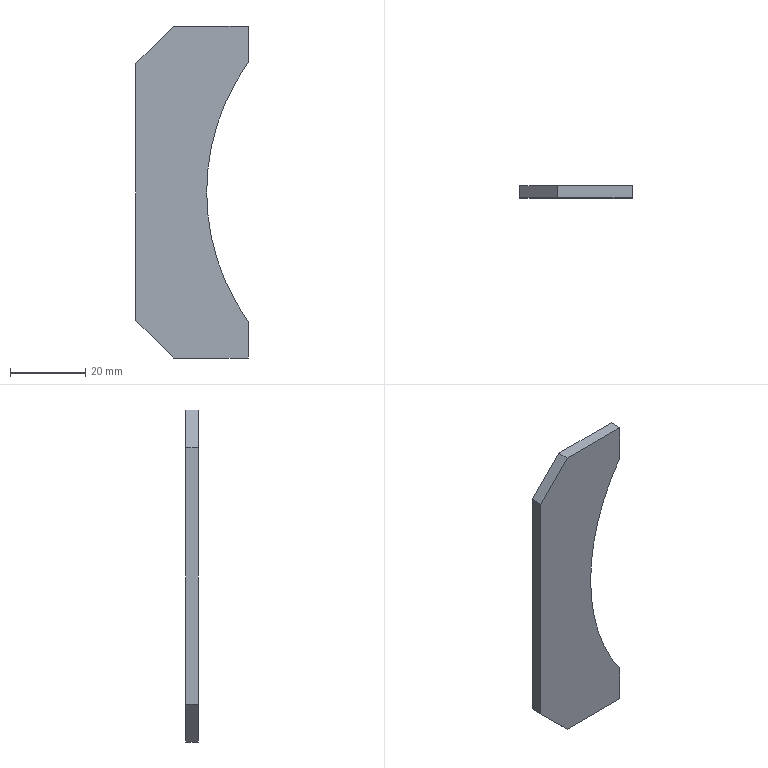Part | SolidWorks | features FlatPattern 1, SMBaseFlange 1, SheetMetal 1 | 1 solid | 10 faces | box 29.8 x 3.2 x 88.1 mm | volume 6438 mm3 | plane 9 | cylinder 1 | commonest cylinder face diameters 118 x1
STEP:
#1=CARTESIAN_POINT('',(0.,0.,9.743));
#2=VERTEX_POINT('',#1);
#3=CARTESIAN_POINT('',(0.,0.,0.));
#4=VERTEX_POINT('',#3);
#5=CARTESIAN_POINT('',(0.,0.,9.743));
#6=DIRECTION('',(0.,0.,-1.));
#7=VECTOR('',#6,1000.);
#8=LINE('',#5,#7);
#9=EDGE_CURVE('',#2,#4,#8,.T.);
#10=ORIENTED_EDGE('',*,*,#9,.F.);
#11=CARTESIAN_POINT('',(0.,-3.2,9.743));
#12=VERTEX_POINT('',#11);
#13=CARTESIAN_POINT('',(0.,-3.2,9.743));
#14=DIRECTION('',(0.,1.,0.));
#15=VECTOR('',#14,1000.);
#16=LINE('',#13,#15);
#17=EDGE_CURVE('',#12,#2,#16,.T.);
#18=ORIENTED_EDGE('',*,*,#17,.F.);
#19=CARTESIAN_POINT('',(0.,-3.2,0.));
#20=VERTEX_POINT('',#19);
#21=CARTESIAN_POINT('',(0.,-3.2,9.743));
#22=DIRECTION('',(0.,0.,-1.));
#23=VECTOR('',#22,1000.);
#24=LINE('',#21,#23);
#25=EDGE_CURVE('',#12,#20,#24,.T.);
#26=ORIENTED_EDGE('',*,*,#25,.T.);
#27=CARTESIAN_POINT('',(0.,-3.2,0.));
#28=DIRECTION('',(0.,1.,0.));
#29=VECTOR('',#28,1000.);
#30=LINE('',#27,#29);
#31=EDGE_CURVE('',#20,#4,#30,.T.);
#32=ORIENTED_EDGE('',*,*,#31,.T.);
#33=EDGE_LOOP('',(#10,#18,#26,#32));
#34=FACE_OUTER_BOUND('',#33,.T.);
#35=CARTESIAN_POINT('',(0.,-3.2,9.743));
#36=DIRECTION('',(1.,0.,0.));
#37=DIRECTION('',(0.,0.,-1.));
#38=AXIS2_PLACEMENT_3D('',#35,#36,#37);
#39=PLANE('',#38);
#40=ADVANCED_FACE('',(#34),#39,.T.);
#41=CARTESIAN_POINT('',(0.,0.,78.357));
#42=VERTEX_POINT('',#41);
#43=CARTESIAN_POINT('',(48.,0.,44.05));
#44=DIRECTION('',(0.,-1.,0.));
#45=DIRECTION('',(0.,0.,1.));
#46=AXIS2_PLACEMENT_3D('',#43,#44,#45);
#47=CIRCLE('',#46,59.);
#48=EDGE_CURVE('',#42,#2,#47,.T.);
#49=ORIENTED_EDGE('',*,*,#48,.F.);
#50=CARTESIAN_POINT('',(0.,-3.2,78.357));
#51=VERTEX_POINT('',#50);
#52=CARTESIAN_POINT('',(0.,-3.2,78.357));
#53=DIRECTION('',(0.,1.,0.));
#54=VECTOR('',#53,1000.);
#55=LINE('',#52,#54);
#56=EDGE_CURVE('',#51,#42,#55,.T.);
#57=ORIENTED_EDGE('',*,*,#56,.F.);
#58=CARTESIAN_POINT('',(48.,-3.2,44.05));
#59=DIRECTION('',(0.,-1.,0.));
#60=DIRECTION('',(0.,0.,1.));
#61=AXIS2_PLACEMENT_3D('',#58,#59,#60);
#62=CIRCLE('',#61,59.);
#63=EDGE_CURVE('',#51,#12,#62,.T.);
#64=ORIENTED_EDGE('',*,*,#63,.T.);
#65=ORIENTED_EDGE('',*,*,#17,.T.);
#66=EDGE_LOOP('',(#49,#57,#64,#65));
#67=FACE_OUTER_BOUND('',#66,.T.);
#68=CARTESIAN_POINT('',(48.,-3.2,44.05));
#69=DIRECTION('',(0.,1.,0.));
#70=DIRECTION('',(0.,0.,1.));
#71=AXIS2_PLACEMENT_3D('',#68,#69,#70);
#72=CYLINDRICAL_SURFACE('',#71,59.);
#73=ADVANCED_FACE('',(#67),#72,.F.);
#74=CARTESIAN_POINT('',(0.,0.,88.1));
#75=VERTEX_POINT('',#74);
#76=CARTESIAN_POINT('',(0.,0.,88.1));
#77=DIRECTION('',(0.,0.,-1.));
#78=VECTOR('',#77,1000.);
#79=LINE('',#76,#78);
#80=EDGE_CURVE('',#75,#42,#79,.T.);
#81=ORIENTED_EDGE('',*,*,#80,.F.);
#82=CARTESIAN_POINT('',(0.,-3.2,88.1));
#83=VERTEX_POINT('',#82);
#84=CARTESIAN_POINT('',(0.,-3.2,88.1));
#85=DIRECTION('',(0.,1.,0.));
#86=VECTOR('',#85,1000.);
#87=LINE('',#84,#86);
#88=EDGE_CURVE('',#83,#75,#87,.T.);
#89=ORIENTED_EDGE('',*,*,#88,.F.);
#90=CARTESIAN_POINT('',(0.,-3.2,88.1));
#91=DIRECTION('',(0.,0.,-1.));
#92=VECTOR('',#91,1000.);
#93=LINE('',#90,#92);
#94=EDGE_CURVE('',#83,#51,#93,.T.);
#95=ORIENTED_EDGE('',*,*,#94,.T.);
#96=ORIENTED_EDGE('',*,*,#56,.T.);
#97=EDGE_LOOP('',(#81,#89,#95,#96));
#98=FACE_OUTER_BOUND('',#97,.T.);
#99=CARTESIAN_POINT('',(0.,-3.2,88.1));
#100=DIRECTION('',(1.,0.,0.));
#101=DIRECTION('',(0.,0.,-1.));
#102=AXIS2_PLACEMENT_3D('',#99,#100,#101);
#103=PLANE('',#102);
#104=ADVANCED_FACE('',(#98),#103,.T.);
#105=CARTESIAN_POINT('',(-19.8,0.,88.1));
#106=VERTEX_POINT('',#105);
#107=CARTESIAN_POINT('',(-19.8,0.,88.1));
#108=DIRECTION('',(1.,0.,0.));
#109=VECTOR('',#108,1000.);
#110=LINE('',#107,#109);
#111=EDGE_CURVE('',#106,#75,#110,.T.);
#112=ORIENTED_EDGE('',*,*,#111,.F.);
#113=CARTESIAN_POINT('',(-19.8,-3.2,88.1));
#114=VERTEX_POINT('',#113);
#115=CARTESIAN_POINT('',(-19.8,-3.2,88.1));
#116=DIRECTION('',(0.,1.,0.));
#117=VECTOR('',#116,1000.);
#118=LINE('',#115,#117);
#119=EDGE_CURVE('',#114,#106,#118,.T.);
#120=ORIENTED_EDGE('',*,*,#119,.F.);
#121=CARTESIAN_POINT('',(-19.8,-3.2,88.1));
#122=DIRECTION('',(1.,0.,0.));
#123=VECTOR('',#122,1000.);
#124=LINE('',#121,#123);
#125=EDGE_CURVE('',#114,#83,#124,.T.);
#126=ORIENTED_EDGE('',*,*,#125,.T.);
#127=ORIENTED_EDGE('',*,*,#88,.T.);
#128=EDGE_LOOP('',(#112,#120,#126,#127));
#129=FACE_OUTER_BOUND('',#128,.T.);
#130=CARTESIAN_POINT('',(-19.8,-3.2,88.1));
#131=DIRECTION('',(0.,0.,1.));
#132=DIRECTION('',(1.,0.,0.));
#133=AXIS2_PLACEMENT_3D('',#130,#131,#132);
#134=PLANE('',#133);
#135=ADVANCED_FACE('',(#129),#134,.T.);
#136=CARTESIAN_POINT('',(-29.8,0.,78.1));
#137=VERTEX_POINT('',#136);
#138=CARTESIAN_POINT('',(-29.8,0.,78.1));
#139=DIRECTION('',(0.7071,0.,0.7071));
#140=VECTOR('',#139,1000.);
#141=LINE('',#138,#140);
#142=EDGE_CURVE('',#137,#106,#141,.T.);
#143=ORIENTED_EDGE('',*,*,#142,.F.);
#144=CARTESIAN_POINT('',(-29.8,-3.2,78.1));
#145=VERTEX_POINT('',#144);
#146=CARTESIAN_POINT('',(-29.8,-3.2,78.1));
#147=DIRECTION('',(0.,1.,0.));
#148=VECTOR('',#147,1000.);
#149=LINE('',#146,#148);
#150=EDGE_CURVE('',#145,#137,#149,.T.);
#151=ORIENTED_EDGE('',*,*,#150,.F.);
#152=CARTESIAN_POINT('',(-29.8,-3.2,78.1));
#153=DIRECTION('',(0.7071,0.,0.7071));
#154=VECTOR('',#153,1000.);
#155=LINE('',#152,#154);
#156=EDGE_CURVE('',#145,#114,#155,.T.);
#157=ORIENTED_EDGE('',*,*,#156,.T.);
#158=ORIENTED_EDGE('',*,*,#119,.T.);
#159=EDGE_LOOP('',(#143,#151,#157,#158));
#160=FACE_OUTER_BOUND('',#159,.T.);
#161=CARTESIAN_POINT('',(-29.8,-3.2,78.1));
#162=DIRECTION('',(-0.7071,0.,0.7071));
#163=DIRECTION('',(0.7071,0.,0.7071));
#164=AXIS2_PLACEMENT_3D('',#161,#162,#163);
#165=PLANE('',#164);
#166=ADVANCED_FACE('',(#160),#165,.T.);
#167=CARTESIAN_POINT('',(-29.8,0.,10.));
#168=VERTEX_POINT('',#167);
#169=CARTESIAN_POINT('',(-29.8,0.,10.));
#170=DIRECTION('',(0.,0.,1.));
#171=VECTOR('',#170,1000.);
#172=LINE('',#169,#171);
#173=EDGE_CURVE('',#168,#137,#172,.T.);
#174=ORIENTED_EDGE('',*,*,#173,.F.);
#175=CARTESIAN_POINT('',(-29.8,-3.2,10.));
#176=VERTEX_POINT('',#175);
#177=CARTESIAN_POINT('',(-29.8,-3.2,10.));
#178=DIRECTION('',(0.,1.,0.));
#179=VECTOR('',#178,1000.);
#180=LINE('',#177,#179);
#181=EDGE_CURVE('',#176,#168,#180,.T.);
#182=ORIENTED_EDGE('',*,*,#181,.F.);
#183=CARTESIAN_POINT('',(-29.8,-3.2,10.));
#184=DIRECTION('',(0.,0.,1.));
#185=VECTOR('',#184,1000.);
#186=LINE('',#183,#185);
#187=EDGE_CURVE('',#176,#145,#186,.T.);
#188=ORIENTED_EDGE('',*,*,#187,.T.);
#189=ORIENTED_EDGE('',*,*,#150,.T.);
#190=EDGE_LOOP('',(#174,#182,#188,#189));
#191=FACE_OUTER_BOUND('',#190,.T.);
#192=CARTESIAN_POINT('',(-29.8,-3.2,10.));
#193=DIRECTION('',(-1.,0.,0.));
#194=DIRECTION('',(0.,0.,1.));
#195=AXIS2_PLACEMENT_3D('',#192,#193,#194);
#196=PLANE('',#195);
#197=ADVANCED_FACE('',(#191),#196,.T.);
#198=CARTESIAN_POINT('',(-19.8,0.,0.));
#199=VERTEX_POINT('',#198);
#200=CARTESIAN_POINT('',(-19.8,0.,0.));
#201=DIRECTION('',(-0.7071,0.,0.7071));
#202=VECTOR('',#201,1000.);
#203=LINE('',#200,#202);
#204=EDGE_CURVE('',#199,#168,#203,.T.);
#205=ORIENTED_EDGE('',*,*,#204,.F.);
#206=CARTESIAN_POINT('',(-19.8,-3.2,0.));
#207=VERTEX_POINT('',#206);
#208=CARTESIAN_POINT('',(-19.8,-3.2,0.));
#209=DIRECTION('',(0.,1.,0.));
#210=VECTOR('',#209,1000.);
#211=LINE('',#208,#210);
#212=EDGE_CURVE('',#207,#199,#211,.T.);
#213=ORIENTED_EDGE('',*,*,#212,.F.);
#214=CARTESIAN_POINT('',(-19.8,-3.2,0.));
#215=DIRECTION('',(-0.7071,0.,0.7071));
#216=VECTOR('',#215,1000.);
#217=LINE('',#214,#216);
#218=EDGE_CURVE('',#207,#176,#217,.T.);
#219=ORIENTED_EDGE('',*,*,#218,.T.);
#220=ORIENTED_EDGE('',*,*,#181,.T.);
#221=EDGE_LOOP('',(#205,#213,#219,#220));
#222=FACE_OUTER_BOUND('',#221,.T.);
#223=CARTESIAN_POINT('',(-19.8,-3.2,0.));
#224=DIRECTION('',(-0.7071,0.,-0.7071));
#225=DIRECTION('',(-0.7071,0.,0.7071));
#226=AXIS2_PLACEMENT_3D('',#223,#224,#225);
#227=PLANE('',#226);
#228=ADVANCED_FACE('',(#222),#227,.T.);
#229=CARTESIAN_POINT('',(0.,0.,0.));
#230=DIRECTION('',(-1.,0.,0.));
#231=VECTOR('',#230,1000.);
#232=LINE('',#229,#231);
#233=EDGE_CURVE('',#4,#199,#232,.T.);
#234=ORIENTED_EDGE('',*,*,#233,.F.);
#235=ORIENTED_EDGE('',*,*,#31,.F.);
#236=CARTESIAN_POINT('',(0.,-3.2,0.));
#237=DIRECTION('',(-1.,0.,0.));
#238=VECTOR('',#237,1000.);
#239=LINE('',#236,#238);
#240=EDGE_CURVE('',#20,#207,#239,.T.);
#241=ORIENTED_EDGE('',*,*,#240,.T.);
#242=ORIENTED_EDGE('',*,*,#212,.T.);
#243=EDGE_LOOP('',(#234,#235,#241,#242));
#244=FACE_OUTER_BOUND('',#243,.T.);
#245=CARTESIAN_POINT('',(0.,-3.2,0.));
#246=DIRECTION('',(0.,0.,-1.));
#247=DIRECTION('',(-1.,0.,0.));
#248=AXIS2_PLACEMENT_3D('',#245,#246,#247);
#249=PLANE('',#248);
#250=ADVANCED_FACE('',(#244),#249,.T.);
#251=ORIENTED_EDGE('',*,*,#25,.F.);
#252=ORIENTED_EDGE('',*,*,#63,.F.);
#253=ORIENTED_EDGE('',*,*,#94,.F.);
#254=ORIENTED_EDGE('',*,*,#125,.F.);
#255=ORIENTED_EDGE('',*,*,#156,.F.);
#256=ORIENTED_EDGE('',*,*,#187,.F.);
#257=ORIENTED_EDGE('',*,*,#218,.F.);
#258=ORIENTED_EDGE('',*,*,#240,.F.);
#259=EDGE_LOOP('',(#251,#252,#253,#254,#255,#256,#257,#258));
#260=FACE_OUTER_BOUND('',#259,.T.);
#261=CARTESIAN_POINT('',(48.,-3.2,44.05));
#262=DIRECTION('',(0.,1.,0.));
#263=DIRECTION('',(0.,0.,1.));
#264=AXIS2_PLACEMENT_3D('',#261,#262,#263);
#265=PLANE('',#264);
#266=ADVANCED_FACE('',(#260),#265,.F.);
#267=ORIENTED_EDGE('',*,*,#9,.T.);
#268=ORIENTED_EDGE('',*,*,#233,.T.);
#269=ORIENTED_EDGE('',*,*,#204,.T.);
#270=ORIENTED_EDGE('',*,*,#173,.T.);
#271=ORIENTED_EDGE('',*,*,#142,.T.);
#272=ORIENTED_EDGE('',*,*,#111,.T.);
#273=ORIENTED_EDGE('',*,*,#80,.T.);
#274=ORIENTED_EDGE('',*,*,#48,.T.);
#275=EDGE_LOOP('',(#267,#268,#269,#270,#271,#272,#273,#274));
#276=FACE_OUTER_BOUND('',#275,.T.);
#277=CARTESIAN_POINT('',(48.,0.,44.05));
#278=DIRECTION('',(0.,1.,0.));
#279=DIRECTION('',(0.,0.,1.));
#280=AXIS2_PLACEMENT_3D('',#277,#278,#279);
#281=PLANE('',#280);
#282=ADVANCED_FACE('',(#276),#281,.T.);
#283=CLOSED_SHELL('',(#40,#73,#104,#135,#166,#197,#228,#250,#266,#282));
#284=MANIFOLD_SOLID_BREP('',#283);
#285=CARTESIAN_POINT('',(0.,0.,0.));
#286=DIRECTION('',(0.,0.,1.));
#287=DIRECTION('',(1.,0.,0.));
#288=AXIS2_PLACEMENT_3D('',#285,#286,#287);
#289=(LENGTH_UNIT()NAMED_UNIT(*)SI_UNIT(.MILLI.,.METRE.));
#290=UNCERTAINTY_MEASURE_WITH_UNIT(LENGTH_MEASURE(0.00001),#289,'','');
#291=(NAMED_UNIT(*)PLANE_ANGLE_UNIT()SI_UNIT($,.RADIAN.));
#292=(NAMED_UNIT(*)SI_UNIT($,.STERADIAN.)SOLID_ANGLE_UNIT());
#293=(GEOMETRIC_REPRESENTATION_CONTEXT(3)GLOBAL_UNCERTAINTY_ASSIGNED_CONTEXT((#290))GLOBAL_UNIT_ASSIGNED_CONTEXT((#289,#291,#292))REPRESENTATION_CONTEXT('',''));
#294=ADVANCED_BREP_SHAPE_REPRESENTATION('',(#284,#288),#293);